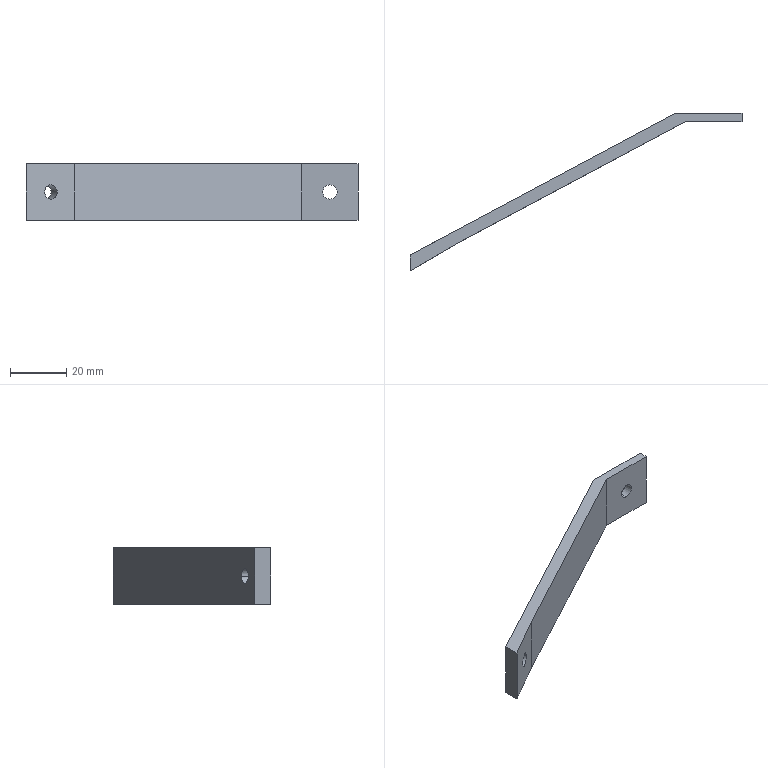Part | STEP file | Front frame | 1 solid | 13 faces | box 118.103 x 56.081 x 20 mm | volume 10734 mm3 | plane 9 | cylinder 4 | commonest cylinder face diameters 5.1 x4
STEP:
#1=CARTESIAN_POINT('',(0.,0.,0.));
#2=DIRECTION('',(0.,0.,1.));
#3=DIRECTION('',(1.,0.,0.));
#4=AXIS2_PLACEMENT_3D('',#1,#2,#3);
#5=CARTESIAN_POINT('',(-91.445,-49.238,10.));
#6=VERTEX_POINT('',#5);
#7=CARTESIAN_POINT('',(-93.677,-45.052,10.));
#8=VERTEX_POINT('',#7);
#9=CARTESIAN_POINT('',(-86.618,-58.288,10.));
#10=DIRECTION('',(-0.4706,0.8824,0.));
#11=VECTOR('',#10,1.);
#12=LINE('',#9,#11);
#13=CARTESIAN_POINT('',(-84.368,-57.088,10.));
#14=DIRECTION('',(-0.4706,0.8824,0.));
#15=DIRECTION('',(-0.8824,-0.4706,0.));
#16=AXIS2_PLACEMENT_3D('',#13,#14,#15);
#17=CYLINDRICAL_SURFACE('',#16,2.55);
#18=CARTESIAN_POINT('',(6.283,0.));
#19=DIRECTION('',(0.,1.));
#20=VECTOR('',#19,1.);
#21=LINE('',#18,#20);
#22=(GEOMETRIC_REPRESENTATION_CONTEXT(2)PARAMETRIC_REPRESENTATION_CONTEXT()REPRESENTATION_CONTEXT('',''));
#23=DEFINITIONAL_REPRESENTATION('',(#21),#22);
#24=PCURVE('',#17,#23);
#25=CARTESIAN_POINT('',(-84.368,-57.088,10.));
#26=DIRECTION('',(-0.4706,0.8824,0.));
#27=DIRECTION('',(-0.8824,-0.4706,0.));
#28=AXIS2_PLACEMENT_3D('',#25,#26,#27);
#29=CYLINDRICAL_SURFACE('',#28,2.55);
#30=CARTESIAN_POINT('',(0.,0.));
#31=DIRECTION('',(0.,1.));
#32=VECTOR('',#31,1.);
#33=LINE('',#30,#32);
#34=(GEOMETRIC_REPRESENTATION_CONTEXT(2)PARAMETRIC_REPRESENTATION_CONTEXT()REPRESENTATION_CONTEXT('',''));
#35=DEFINITIONAL_REPRESENTATION('',(#33),#34);
#36=PCURVE('',#29,#35);
#37=SURFACE_CURVE('',#12,(#24,#36),.PCURVE_S1.);
#38=EDGE_CURVE('',#6,#8,#37,.T.);
#39=ORIENTED_EDGE('',*,*,#38,.T.);
#40=CARTESIAN_POINT('',(-89.177,-42.652,10.));
#41=VERTEX_POINT('',#40);
#42=CARTESIAN_POINT('',(-91.427,-43.852,10.));
#43=DIRECTION('',(-0.4706,0.8824,0.));
#44=DIRECTION('',(-0.8824,-0.4706,0.));
#45=AXIS2_PLACEMENT_3D('',#42,#43,#44);
#46=CIRCLE('',#45,2.55);
#47=CARTESIAN_POINT('',(0.,15.));
#48=DIRECTION('',(1.,0.));
#49=VECTOR('',#48,1.);
#50=LINE('',#47,#49);
#51=(GEOMETRIC_REPRESENTATION_CONTEXT(2)PARAMETRIC_REPRESENTATION_CONTEXT()REPRESENTATION_CONTEXT('',''));
#52=DEFINITIONAL_REPRESENTATION('',(#50),#51);
#53=PCURVE('',#17,#52);
#54=CARTESIAN_POINT('',(-98.103,-47.412,133.001));
#55=DIRECTION('',(-0.4706,0.8824,0.));
#56=DIRECTION('',(-0.8824,-0.4706,0.));
#57=AXIS2_PLACEMENT_3D('',#54,#55,#56);
#58=PLANE('',#57);
#59=CARTESIAN_POINT('',(-7.566,-123.001));
#60=DIRECTION('',(1.,0.));
#61=AXIS2_PLACEMENT_2D('',#59,#60);
#62=CIRCLE('',#61,2.55);
#63=(GEOMETRIC_REPRESENTATION_CONTEXT(2)PARAMETRIC_REPRESENTATION_CONTEXT()REPRESENTATION_CONTEXT('',''));
#64=DEFINITIONAL_REPRESENTATION('',(#62),#63);
#65=PCURVE('',#58,#64);
#66=SURFACE_CURVE('',#46,(#53,#65),.PCURVE_S1.);
#67=EDGE_CURVE('',#41,#8,#66,.T.);
#68=ORIENTED_EDGE('',*,*,#67,.F.);
#69=CARTESIAN_POINT('',(-87.026,-46.686,10.));
#70=VERTEX_POINT('',#69);
#71=CARTESIAN_POINT('',(-82.118,-55.888,10.));
#72=DIRECTION('',(-0.4706,0.8824,0.));
#73=VECTOR('',#72,1.);
#74=LINE('',#71,#73);
#75=CARTESIAN_POINT('',(3.142,0.));
#76=DIRECTION('',(0.,1.));
#77=VECTOR('',#76,1.);
#78=LINE('',#75,#77);
#79=(GEOMETRIC_REPRESENTATION_CONTEXT(2)PARAMETRIC_REPRESENTATION_CONTEXT()REPRESENTATION_CONTEXT('',''));
#80=DEFINITIONAL_REPRESENTATION('',(#78),#79);
#81=PCURVE('',#17,#80);
#82=CARTESIAN_POINT('',(3.142,0.));
#83=DIRECTION('',(0.,1.));
#84=VECTOR('',#83,1.);
#85=LINE('',#82,#84);
#86=(GEOMETRIC_REPRESENTATION_CONTEXT(2)PARAMETRIC_REPRESENTATION_CONTEXT()REPRESENTATION_CONTEXT('',''));
#87=DEFINITIONAL_REPRESENTATION('',(#85),#86);
#88=PCURVE('',#29,#87);
#89=SURFACE_CURVE('',#74,(#81,#88),.PCURVE_S1.);
#90=EDGE_CURVE('',#70,#41,#89,.T.);
#91=ORIENTED_EDGE('',*,*,#90,.F.);
#92=CARTESIAN_POINT('',(-91.445,-49.238,10.));
#93=CARTESIAN_POINT('',(-91.445,-49.238,4.9));
#94=CARTESIAN_POINT('',(-87.026,-46.686,4.9));
#95=CARTESIAN_POINT('',(-87.026,-46.686,10.));
#96=(BOUNDED_CURVE()B_SPLINE_CURVE(3,(#92,#93,#94,#95),.UNSPECIFIED.,.F.,.F.)B_SPLINE_CURVE_WITH_KNOTS((4,4),(3.142,6.283),.PIECEWISE_BEZIER_KNOTS.)CURVE()GEOMETRIC_REPRESENTATION_ITEM()RATIONAL_B_SPLINE_CURVE((1.,0.3333,0.3333,1.))REPRESENTATION_ITEM(''));
#97=CARTESIAN_POINT('',(6.283,10.257));
#98=CARTESIAN_POINT('',(6.253,10.257));
#99=CARTESIAN_POINT('',(6.19,10.257));
#100=CARTESIAN_POINT('',(6.085,10.258));
#101=CARTESIAN_POINT('',(5.972,10.26));
#102=CARTESIAN_POINT('',(5.848,10.264));
#103=CARTESIAN_POINT('',(5.713,10.27));
#104=CARTESIAN_POINT('',(5.567,10.277));
#105=CARTESIAN_POINT('',(5.412,10.287));
#106=CARTESIAN_POINT('',(5.246,10.298));
#107=CARTESIAN_POINT('',(5.073,10.312));
#108=CARTESIAN_POINT('',(4.894,10.327));
#109=CARTESIAN_POINT('',(4.712,10.342));
#110=CARTESIAN_POINT('',(4.531,10.358));
#111=CARTESIAN_POINT('',(4.352,10.373));
#112=CARTESIAN_POINT('',(4.179,10.386));
#113=CARTESIAN_POINT('',(4.013,10.398));
#114=CARTESIAN_POINT('',(3.857,10.407));
#115=CARTESIAN_POINT('',(3.712,10.415));
#116=CARTESIAN_POINT('',(3.577,10.42));
#117=CARTESIAN_POINT('',(3.453,10.424));
#118=CARTESIAN_POINT('',(3.339,10.427));
#119=CARTESIAN_POINT('',(3.235,10.428));
#120=CARTESIAN_POINT('',(3.172,10.428));
#121=CARTESIAN_POINT('',(3.142,10.428));
#122=B_SPLINE_CURVE_WITH_KNOTS('',3,(#97,#98,#99,#100,#101,#102,#103,#104,#105,#106,#107,#108,#109,#110,#111,#112,#113,#114,#115,#116,#117,#118,#119,#120,#121),.UNSPECIFIED.,.F.,.F.,(4,1,1,1,1,1,1,1,1,1,1,1,1,1,1,1,1,1,1,1,1,1,4),(3.142,3.284,3.427,3.57,3.713,3.856,3.998,4.141,4.284,4.427,4.57,4.712,4.855,4.998,5.141,5.284,5.426,5.569,5.712,5.855,5.998,6.14,6.283),.QUASI_UNIFORM_KNOTS.);
#123=(GEOMETRIC_REPRESENTATION_CONTEXT(2)PARAMETRIC_REPRESENTATION_CONTEXT()REPRESENTATION_CONTEXT('',''));
#124=DEFINITIONAL_REPRESENTATION('',(#122),#123);
#125=PCURVE('',#17,#124);
#126=CARTESIAN_POINT('',(-80.782,-43.081,133.001));
#127=DIRECTION('',(0.5,-0.866,0.));
#128=DIRECTION('',(0.866,0.5,0.));
#129=AXIS2_PLACEMENT_3D('',#126,#127,#128);
#130=PLANE('',#129);
#131=CARTESIAN_POINT('',(-12.312,-123.001));
#132=CARTESIAN_POINT('',(-12.312,-128.101));
#133=CARTESIAN_POINT('',(-7.209,-128.101));
#134=CARTESIAN_POINT('',(-7.209,-123.001));
#135=(BOUNDED_CURVE()B_SPLINE_CURVE(3,(#131,#132,#133,#134),.UNSPECIFIED.,.F.,.F.)B_SPLINE_CURVE_WITH_KNOTS((4,4),(3.142,6.283),.PIECEWISE_BEZIER_KNOTS.)CURVE()GEOMETRIC_REPRESENTATION_ITEM()RATIONAL_B_SPLINE_CURVE((1.,0.3333,0.3333,1.))REPRESENTATION_ITEM(''));
#136=(GEOMETRIC_REPRESENTATION_CONTEXT(2)PARAMETRIC_REPRESENTATION_CONTEXT()REPRESENTATION_CONTEXT('',''));
#137=DEFINITIONAL_REPRESENTATION('',(#135),#136);
#138=PCURVE('',#130,#137);
#139=SURFACE_CURVE('',#96,(#125,#138),.PCURVE_S1.);
#140=EDGE_CURVE('',#6,#70,#139,.T.);
#141=ORIENTED_EDGE('',*,*,#140,.F.);
#142=EDGE_LOOP('',(#39,#68,#91,#141));
#143=FACE_BOUND('',#142,.F.);
#144=ADVANCED_FACE('',(#143),#17,.F.);
#145=CARTESIAN_POINT('',(10.,3.,7.45));
#146=VERTEX_POINT('',#145);
#147=CARTESIAN_POINT('',(10.,0.,7.45));
#148=VERTEX_POINT('',#147);
#149=CARTESIAN_POINT('',(10.,3.,7.45));
#150=DIRECTION('',(0.,-1.,0.));
#151=VECTOR('',#150,1.);
#152=LINE('',#149,#151);
#153=CARTESIAN_POINT('',(10.,3.,10.));
#154=DIRECTION('',(0.,-1.,0.));
#155=DIRECTION('',(0.,0.,-1.));
#156=AXIS2_PLACEMENT_3D('',#153,#154,#155);
#157=CYLINDRICAL_SURFACE('',#156,2.55);
#158=CARTESIAN_POINT('',(6.283,0.));
#159=DIRECTION('',(0.,1.));
#160=VECTOR('',#159,1.);
#161=LINE('',#158,#160);
#162=(GEOMETRIC_REPRESENTATION_CONTEXT(2)PARAMETRIC_REPRESENTATION_CONTEXT()REPRESENTATION_CONTEXT('',''));
#163=DEFINITIONAL_REPRESENTATION('',(#161),#162);
#164=PCURVE('',#157,#163);
#165=CARTESIAN_POINT('',(10.,3.,10.));
#166=DIRECTION('',(0.,-1.,0.));
#167=DIRECTION('',(0.,0.,-1.));
#168=AXIS2_PLACEMENT_3D('',#165,#166,#167);
#169=CYLINDRICAL_SURFACE('',#168,2.55);
#170=CARTESIAN_POINT('',(0.,0.));
#171=DIRECTION('',(0.,1.));
#172=VECTOR('',#171,1.);
#173=LINE('',#170,#172);
#174=(GEOMETRIC_REPRESENTATION_CONTEXT(2)PARAMETRIC_REPRESENTATION_CONTEXT()REPRESENTATION_CONTEXT('',''));
#175=DEFINITIONAL_REPRESENTATION('',(#173),#174);
#176=PCURVE('',#169,#175);
#177=SURFACE_CURVE('',#152,(#164,#176),.PCURVE_S1.);
#178=EDGE_CURVE('',#146,#148,#177,.T.);
#179=ORIENTED_EDGE('',*,*,#178,.T.);
#180=CARTESIAN_POINT('',(10.,0.,12.55));
#181=VERTEX_POINT('',#180);
#182=CARTESIAN_POINT('',(10.,0.,10.));
#183=DIRECTION('',(0.,1.,0.));
#184=DIRECTION('',(0.,0.,1.));
#185=AXIS2_PLACEMENT_3D('',#182,#183,#184);
#186=CIRCLE('',#185,2.55);
#187=CARTESIAN_POINT('',(9.425,3.));
#188=DIRECTION('',(-1.,0.));
#189=VECTOR('',#188,1.);
#190=LINE('',#187,#189);
#191=(GEOMETRIC_REPRESENTATION_CONTEXT(2)PARAMETRIC_REPRESENTATION_CONTEXT()REPRESENTATION_CONTEXT('',''));
#192=DEFINITIONAL_REPRESENTATION('',(#190),#191);
#193=PCURVE('',#157,#192);
#194=CARTESIAN_POINT('',(0.,0.,0.));
#195=DIRECTION('',(0.,1.,0.));
#196=DIRECTION('',(0.,0.,1.));
#197=AXIS2_PLACEMENT_3D('',#194,#195,#196);
#198=PLANE('',#197);
#199=CARTESIAN_POINT('',(10.,10.));
#200=DIRECTION('',(1.,0.));
#201=AXIS2_PLACEMENT_2D('',#199,#200);
#202=CIRCLE('',#201,2.55);
#203=(GEOMETRIC_REPRESENTATION_CONTEXT(2)PARAMETRIC_REPRESENTATION_CONTEXT()REPRESENTATION_CONTEXT('',''));
#204=DEFINITIONAL_REPRESENTATION('',(#202),#203);
#205=PCURVE('',#198,#204);
#206=SURFACE_CURVE('',#186,(#193,#205),.PCURVE_S1.);
#207=EDGE_CURVE('',#148,#181,#206,.T.);
#208=ORIENTED_EDGE('',*,*,#207,.T.);
#209=CARTESIAN_POINT('',(10.,3.,12.55));
#210=VERTEX_POINT('',#209);
#211=CARTESIAN_POINT('',(10.,3.,12.55));
#212=DIRECTION('',(0.,-1.,0.));
#213=VECTOR('',#212,1.);
#214=LINE('',#211,#213);
#215=CARTESIAN_POINT('',(3.142,0.));
#216=DIRECTION('',(0.,1.));
#217=VECTOR('',#216,1.);
#218=LINE('',#215,#217);
#219=(GEOMETRIC_REPRESENTATION_CONTEXT(2)PARAMETRIC_REPRESENTATION_CONTEXT()REPRESENTATION_CONTEXT('',''));
#220=DEFINITIONAL_REPRESENTATION('',(#218),#219);
#221=PCURVE('',#157,#220);
#222=CARTESIAN_POINT('',(3.142,0.));
#223=DIRECTION('',(0.,1.));
#224=VECTOR('',#223,1.);
#225=LINE('',#222,#224);
#226=(GEOMETRIC_REPRESENTATION_CONTEXT(2)PARAMETRIC_REPRESENTATION_CONTEXT()REPRESENTATION_CONTEXT('',''));
#227=DEFINITIONAL_REPRESENTATION('',(#225),#226);
#228=PCURVE('',#169,#227);
#229=SURFACE_CURVE('',#214,(#221,#228),.PCURVE_S1.);
#230=EDGE_CURVE('',#210,#181,#229,.T.);
#231=ORIENTED_EDGE('',*,*,#230,.F.);
#232=CARTESIAN_POINT('',(10.,3.,10.));
#233=DIRECTION('',(0.,1.,0.));
#234=DIRECTION('',(0.,0.,1.));
#235=AXIS2_PLACEMENT_3D('',#232,#233,#234);
#236=CIRCLE('',#235,2.55);
#237=CARTESIAN_POINT('',(9.425,0.));
#238=DIRECTION('',(-1.,0.));
#239=VECTOR('',#238,1.);
#240=LINE('',#237,#239);
#241=(GEOMETRIC_REPRESENTATION_CONTEXT(2)PARAMETRIC_REPRESENTATION_CONTEXT()REPRESENTATION_CONTEXT('',''));
#242=DEFINITIONAL_REPRESENTATION('',(#240),#241);
#243=PCURVE('',#157,#242);
#244=CARTESIAN_POINT('',(0.,3.,0.));
#245=DIRECTION('',(0.,1.,0.));
#246=DIRECTION('',(0.,0.,1.));
#247=AXIS2_PLACEMENT_3D('',#244,#245,#246);
#248=PLANE('',#247);
#249=CARTESIAN_POINT('',(10.,10.));
#250=DIRECTION('',(1.,0.));
#251=AXIS2_PLACEMENT_2D('',#249,#250);
#252=CIRCLE('',#251,2.55);
#253=(GEOMETRIC_REPRESENTATION_CONTEXT(2)PARAMETRIC_REPRESENTATION_CONTEXT()REPRESENTATION_CONTEXT('',''));
#254=DEFINITIONAL_REPRESENTATION('',(#252),#253);
#255=PCURVE('',#248,#254);
#256=SURFACE_CURVE('',#236,(#243,#255),.PCURVE_S1.);
#257=EDGE_CURVE('',#146,#210,#256,.T.);
#258=ORIENTED_EDGE('',*,*,#257,.F.);
#259=EDGE_LOOP('',(#179,#208,#231,#258));
#260=FACE_BOUND('',#259,.F.);
#261=ADVANCED_FACE('',(#260),#157,.F.);
#262=CARTESIAN_POINT('',(20.,3.,0.));
#263=VERTEX_POINT('',#262);
#264=CARTESIAN_POINT('',(-3.574,3.,0.));
#265=VERTEX_POINT('',#264);
#266=CARTESIAN_POINT('',(0.,3.,0.));
#267=DIRECTION('',(-1.,0.,0.));
#268=VECTOR('',#267,1.);
#269=LINE('',#266,#268);
#270=CARTESIAN_POINT('',(0.,0.));
#271=DIRECTION('',(0.,-1.));
#272=VECTOR('',#271,1.);
#273=LINE('',#270,#272);
#274=(GEOMETRIC_REPRESENTATION_CONTEXT(2)PARAMETRIC_REPRESENTATION_CONTEXT()REPRESENTATION_CONTEXT('',''));
#275=DEFINITIONAL_REPRESENTATION('',(#273),#274);
#276=PCURVE('',#248,#275);
#277=CARTESIAN_POINT('',(0.,3.,0.));
#278=DIRECTION('',(0.,0.,1.));
#279=DIRECTION('',(1.,0.,0.));
#280=AXIS2_PLACEMENT_3D('',#277,#278,#279);
#281=PLANE('',#280);
#282=CARTESIAN_POINT('',(0.,0.));
#283=DIRECTION('',(-1.,0.));
#284=VECTOR('',#283,1.);
#285=LINE('',#282,#284);
#286=(GEOMETRIC_REPRESENTATION_CONTEXT(2)PARAMETRIC_REPRESENTATION_CONTEXT()REPRESENTATION_CONTEXT('',''));
#287=DEFINITIONAL_REPRESENTATION('',(#285),#286);
#288=PCURVE('',#281,#287);
#289=SURFACE_CURVE('',#269,(#276,#288),.PCURVE_S1.);
#290=EDGE_CURVE('',#263,#265,#289,.T.);
#291=ORIENTED_EDGE('',*,*,#290,.T.);
#292=CARTESIAN_POINT('',(-3.574,3.,20.));
#293=VERTEX_POINT('',#292);
#294=CARTESIAN_POINT('',(-3.574,3.,133.001));
#295=DIRECTION('',(0.,0.,-1.));
#296=VECTOR('',#295,1.);
#297=LINE('',#294,#296);
#298=CARTESIAN_POINT('',(133.001,-3.574));
#299=DIRECTION('',(-1.,0.));
#300=VECTOR('',#299,1.);
#301=LINE('',#298,#300);
#302=(GEOMETRIC_REPRESENTATION_CONTEXT(2)PARAMETRIC_REPRESENTATION_CONTEXT()REPRESENTATION_CONTEXT('',''));
#303=DEFINITIONAL_REPRESENTATION('',(#301),#302);
#304=PCURVE('',#248,#303);
#305=CARTESIAN_POINT('',(-107.131,0.));
#306=DIRECTION('',(0.,-1.));
#307=VECTOR('',#306,1.);
#308=LINE('',#305,#307);
#309=(GEOMETRIC_REPRESENTATION_CONTEXT(2)PARAMETRIC_REPRESENTATION_CONTEXT()REPRESENTATION_CONTEXT('',''));
#310=DEFINITIONAL_REPRESENTATION('',(#308),#309);
#311=PCURVE('',#58,#310);
#312=SURFACE_CURVE('',#297,(#304,#311),.PCURVE_S1.);
#313=EDGE_CURVE('',#293,#265,#312,.T.);
#314=ORIENTED_EDGE('',*,*,#313,.F.);
#315=CARTESIAN_POINT('',(20.,3.,20.));
#316=VERTEX_POINT('',#315);
#317=CARTESIAN_POINT('',(0.,3.,20.));
#318=DIRECTION('',(1.,0.,0.));
#319=VECTOR('',#318,1.);
#320=LINE('',#317,#319);
#321=CARTESIAN_POINT('',(20.,0.));
#322=DIRECTION('',(0.,1.));
#323=VECTOR('',#322,1.);
#324=LINE('',#321,#323);
#325=(GEOMETRIC_REPRESENTATION_CONTEXT(2)PARAMETRIC_REPRESENTATION_CONTEXT()REPRESENTATION_CONTEXT('',''));
#326=DEFINITIONAL_REPRESENTATION('',(#324),#325);
#327=PCURVE('',#248,#326);
#328=CARTESIAN_POINT('',(0.,3.,20.));
#329=DIRECTION('',(0.,0.,-1.));
#330=DIRECTION('',(-1.,0.,0.));
#331=AXIS2_PLACEMENT_3D('',#328,#329,#330);
#332=PLANE('',#331);
#333=CARTESIAN_POINT('',(0.,0.));
#334=DIRECTION('',(-1.,0.));
#335=VECTOR('',#334,1.);
#336=LINE('',#333,#335);
#337=(GEOMETRIC_REPRESENTATION_CONTEXT(2)PARAMETRIC_REPRESENTATION_CONTEXT()REPRESENTATION_CONTEXT('',''));
#338=DEFINITIONAL_REPRESENTATION('',(#336),#337);
#339=PCURVE('',#332,#338);
#340=SURFACE_CURVE('',#320,(#327,#339),.PCURVE_S1.);
#341=EDGE_CURVE('',#293,#316,#340,.T.);
#342=ORIENTED_EDGE('',*,*,#341,.T.);
#343=CARTESIAN_POINT('',(20.,3.,0.));
#344=DIRECTION('',(0.,0.,-1.));
#345=VECTOR('',#344,1.);
#346=LINE('',#343,#345);
#347=CARTESIAN_POINT('',(0.,20.));
#348=DIRECTION('',(-1.,0.));
#349=VECTOR('',#348,1.);
#350=LINE('',#347,#349);
#351=(GEOMETRIC_REPRESENTATION_CONTEXT(2)PARAMETRIC_REPRESENTATION_CONTEXT()REPRESENTATION_CONTEXT('',''));
#352=DEFINITIONAL_REPRESENTATION('',(#350),#351);
#353=PCURVE('',#248,#352);
#354=CARTESIAN_POINT('',(20.,3.,0.));
#355=DIRECTION('',(-1.,0.,0.));
#356=DIRECTION('',(0.,0.,1.));
#357=AXIS2_PLACEMENT_3D('',#354,#355,#356);
#358=PLANE('',#357);
#359=CARTESIAN_POINT('',(0.,0.));
#360=DIRECTION('',(-1.,0.));
#361=VECTOR('',#360,1.);
#362=LINE('',#359,#361);
#363=(GEOMETRIC_REPRESENTATION_CONTEXT(2)PARAMETRIC_REPRESENTATION_CONTEXT()REPRESENTATION_CONTEXT('',''));
#364=DEFINITIONAL_REPRESENTATION('',(#362),#363);
#365=PCURVE('',#358,#364);
#366=SURFACE_CURVE('',#346,(#353,#365),.PCURVE_S1.);
#367=EDGE_CURVE('',#316,#263,#366,.T.);
#368=ORIENTED_EDGE('',*,*,#367,.T.);
#369=EDGE_LOOP('',(#291,#314,#342,#368));
#370=FACE_BOUND('',#369,.T.);
#371=ORIENTED_EDGE('',*,*,#257,.F.);
#372=CARTESIAN_POINT('',(10.,3.,10.));
#373=DIRECTION('',(0.,1.,0.));
#374=DIRECTION('',(0.,0.,1.));
#375=AXIS2_PLACEMENT_3D('',#372,#373,#374);
#376=CIRCLE('',#375,2.55);
#377=CARTESIAN_POINT('',(10.,10.));
#378=DIRECTION('',(1.,0.));
#379=AXIS2_PLACEMENT_2D('',#377,#378);
#380=CIRCLE('',#379,2.55);
#381=(GEOMETRIC_REPRESENTATION_CONTEXT(2)PARAMETRIC_REPRESENTATION_CONTEXT()REPRESENTATION_CONTEXT('',''));
#382=DEFINITIONAL_REPRESENTATION('',(#380),#381);
#383=PCURVE('',#248,#382);
#384=CARTESIAN_POINT('',(3.142,0.));
#385=DIRECTION('',(-1.,0.));
#386=VECTOR('',#385,1.);
#387=LINE('',#384,#386);
#388=(GEOMETRIC_REPRESENTATION_CONTEXT(2)PARAMETRIC_REPRESENTATION_CONTEXT()REPRESENTATION_CONTEXT('',''));
#389=DEFINITIONAL_REPRESENTATION('',(#387),#388);
#390=PCURVE('',#169,#389);
#391=SURFACE_CURVE('',#376,(#383,#390),.PCURVE_S1.);
#392=EDGE_CURVE('',#210,#146,#391,.T.);
#393=ORIENTED_EDGE('',*,*,#392,.F.);
#394=EDGE_LOOP('',(#371,#393));
#395=FACE_BOUND('',#394,.T.);
#396=ADVANCED_FACE('',(#370,#395),#248,.T.);
#397=CARTESIAN_POINT('',(0.,0.,0.));
#398=VERTEX_POINT('',#397);
#399=CARTESIAN_POINT('',(0.,0.,20.));
#400=VERTEX_POINT('',#399);
#401=CARTESIAN_POINT('',(0.,0.,0.));
#402=DIRECTION('',(0.,0.,1.));
#403=VECTOR('',#402,1.);
#404=LINE('',#401,#403);
#405=CARTESIAN_POINT('',(0.,0.));
#406=DIRECTION('',(1.,0.));
#407=VECTOR('',#406,1.);
#408=LINE('',#405,#407);
#409=(GEOMETRIC_REPRESENTATION_CONTEXT(2)PARAMETRIC_REPRESENTATION_CONTEXT()REPRESENTATION_CONTEXT('',''));
#410=DEFINITIONAL_REPRESENTATION('',(#408),#409);
#411=PCURVE('',#198,#410);
#412=CARTESIAN_POINT('',(0.,0.,133.001));
#413=DIRECTION('',(0.4706,-0.8824,0.));
#414=DIRECTION('',(0.8824,0.4706,0.));
#415=AXIS2_PLACEMENT_3D('',#412,#413,#414);
#416=PLANE('',#415);
#417=CARTESIAN_POINT('',(0.,-133.001));
#418=DIRECTION('',(0.,1.));
#419=VECTOR('',#418,1.);
#420=LINE('',#417,#419);
#421=(GEOMETRIC_REPRESENTATION_CONTEXT(2)PARAMETRIC_REPRESENTATION_CONTEXT()REPRESENTATION_CONTEXT('',''));
#422=DEFINITIONAL_REPRESENTATION('',(#420),#421);
#423=PCURVE('',#416,#422);
#424=SURFACE_CURVE('',#404,(#411,#423),.PCURVE_S1.);
#425=EDGE_CURVE('',#398,#400,#424,.T.);
#426=ORIENTED_EDGE('',*,*,#425,.F.);
#427=CARTESIAN_POINT('',(20.,0.,0.));
#428=VERTEX_POINT('',#427);
#429=CARTESIAN_POINT('',(0.,0.,0.));
#430=DIRECTION('',(-1.,0.,0.));
#431=VECTOR('',#430,1.);
#432=LINE('',#429,#431);
#433=CARTESIAN_POINT('',(0.,0.));
#434=DIRECTION('',(0.,-1.));
#435=VECTOR('',#434,1.);
#436=LINE('',#433,#435);
#437=(GEOMETRIC_REPRESENTATION_CONTEXT(2)PARAMETRIC_REPRESENTATION_CONTEXT()REPRESENTATION_CONTEXT('',''));
#438=DEFINITIONAL_REPRESENTATION('',(#436),#437);
#439=PCURVE('',#198,#438);
#440=CARTESIAN_POINT('',(0.,-3.));
#441=DIRECTION('',(-1.,0.));
#442=VECTOR('',#441,1.);
#443=LINE('',#440,#442);
#444=(GEOMETRIC_REPRESENTATION_CONTEXT(2)PARAMETRIC_REPRESENTATION_CONTEXT()REPRESENTATION_CONTEXT('',''));
#445=DEFINITIONAL_REPRESENTATION('',(#443),#444);
#446=PCURVE('',#281,#445);
#447=SURFACE_CURVE('',#432,(#439,#446),.PCURVE_S1.);
#448=EDGE_CURVE('',#428,#398,#447,.T.);
#449=ORIENTED_EDGE('',*,*,#448,.F.);
#450=CARTESIAN_POINT('',(20.,0.,20.));
#451=VERTEX_POINT('',#450);
#452=CARTESIAN_POINT('',(20.,0.,0.));
#453=DIRECTION('',(0.,0.,-1.));
#454=VECTOR('',#453,1.);
#455=LINE('',#452,#454);
#456=CARTESIAN_POINT('',(0.,20.));
#457=DIRECTION('',(-1.,0.));
#458=VECTOR('',#457,1.);
#459=LINE('',#456,#458);
#460=(GEOMETRIC_REPRESENTATION_CONTEXT(2)PARAMETRIC_REPRESENTATION_CONTEXT()REPRESENTATION_CONTEXT('',''));
#461=DEFINITIONAL_REPRESENTATION('',(#459),#460);
#462=PCURVE('',#198,#461);
#463=CARTESIAN_POINT('',(0.,-3.));
#464=DIRECTION('',(-1.,0.));
#465=VECTOR('',#464,1.);
#466=LINE('',#463,#465);
#467=(GEOMETRIC_REPRESENTATION_CONTEXT(2)PARAMETRIC_REPRESENTATION_CONTEXT()REPRESENTATION_CONTEXT('',''));
#468=DEFINITIONAL_REPRESENTATION('',(#466),#467);
#469=PCURVE('',#358,#468);
#470=SURFACE_CURVE('',#455,(#462,#469),.PCURVE_S1.);
#471=EDGE_CURVE('',#451,#428,#470,.T.);
#472=ORIENTED_EDGE('',*,*,#471,.F.);
#473=CARTESIAN_POINT('',(0.,0.,20.));
#474=DIRECTION('',(1.,0.,0.));
#475=VECTOR('',#474,1.);
#476=LINE('',#473,#475);
#477=CARTESIAN_POINT('',(20.,0.));
#478=DIRECTION('',(0.,1.));
#479=VECTOR('',#478,1.);
#480=LINE('',#477,#479);
#481=(GEOMETRIC_REPRESENTATION_CONTEXT(2)PARAMETRIC_REPRESENTATION_CONTEXT()REPRESENTATION_CONTEXT('',''));
#482=DEFINITIONAL_REPRESENTATION('',(#480),#481);
#483=PCURVE('',#198,#482);
#484=CARTESIAN_POINT('',(0.,-3.));
#485=DIRECTION('',(-1.,0.));
#486=VECTOR('',#485,1.);
#487=LINE('',#484,#486);
#488=(GEOMETRIC_REPRESENTATION_CONTEXT(2)PARAMETRIC_REPRESENTATION_CONTEXT()REPRESENTATION_CONTEXT('',''));
#489=DEFINITIONAL_REPRESENTATION('',(#487),#488);
#490=PCURVE('',#332,#489);
#491=SURFACE_CURVE('',#476,(#483,#490),.PCURVE_S1.);
#492=EDGE_CURVE('',#400,#451,#491,.T.);
#493=ORIENTED_EDGE('',*,*,#492,.F.);
#494=EDGE_LOOP('',(#426,#449,#472,#493));
#495=FACE_BOUND('',#494,.T.);
#496=ORIENTED_EDGE('',*,*,#207,.T.);
#497=CARTESIAN_POINT('',(10.,0.,10.));
#498=DIRECTION('',(0.,1.,0.));
#499=DIRECTION('',(0.,0.,1.));
#500=AXIS2_PLACEMENT_3D('',#497,#498,#499);
#501=CIRCLE('',#500,2.55);
#502=CARTESIAN_POINT('',(10.,10.));
#503=DIRECTION('',(1.,0.));
#504=AXIS2_PLACEMENT_2D('',#502,#503);
#505=CIRCLE('',#504,2.55);
#506=(GEOMETRIC_REPRESENTATION_CONTEXT(2)PARAMETRIC_REPRESENTATION_CONTEXT()REPRESENTATION_CONTEXT('',''));
#507=DEFINITIONAL_REPRESENTATION('',(#505),#506);
#508=PCURVE('',#198,#507);
#509=CARTESIAN_POINT('',(3.142,3.));
#510=DIRECTION('',(-1.,0.));
#511=VECTOR('',#510,1.);
#512=LINE('',#509,#511);
#513=(GEOMETRIC_REPRESENTATION_CONTEXT(2)PARAMETRIC_REPRESENTATION_CONTEXT()REPRESENTATION_CONTEXT('',''));
#514=DEFINITIONAL_REPRESENTATION('',(#512),#513);
#515=PCURVE('',#169,#514);
#516=SURFACE_CURVE('',#501,(#508,#515),.PCURVE_S1.);
#517=EDGE_CURVE('',#181,#148,#516,.T.);
#518=ORIENTED_EDGE('',*,*,#517,.T.);
#519=EDGE_LOOP('',(#496,#518));
#520=FACE_BOUND('',#519,.T.);
#521=ADVANCED_FACE('',(#495,#520),#198,.F.);
#522=ORIENTED_EDGE('',*,*,#492,.T.);
#523=CARTESIAN_POINT('',(20.,3.,20.));
#524=DIRECTION('',(0.,-1.,0.));
#525=VECTOR('',#524,1.);
#526=LINE('',#523,#525);
#527=CARTESIAN_POINT('',(-20.,0.));
#528=DIRECTION('',(0.,-1.));
#529=VECTOR('',#528,1.);
#530=LINE('',#527,#529);
#531=(GEOMETRIC_REPRESENTATION_CONTEXT(2)PARAMETRIC_REPRESENTATION_CONTEXT()REPRESENTATION_CONTEXT('',''));
#532=DEFINITIONAL_REPRESENTATION('',(#530),#531);
#533=PCURVE('',#332,#532);
#534=CARTESIAN_POINT('',(20.,0.));
#535=DIRECTION('',(0.,-1.));
#536=VECTOR('',#535,1.);
#537=LINE('',#534,#536);
#538=(GEOMETRIC_REPRESENTATION_CONTEXT(2)PARAMETRIC_REPRESENTATION_CONTEXT()REPRESENTATION_CONTEXT('',''));
#539=DEFINITIONAL_REPRESENTATION('',(#537),#538);
#540=PCURVE('',#358,#539);
#541=SURFACE_CURVE('',#526,(#533,#540),.PCURVE_S1.);
#542=EDGE_CURVE('',#316,#451,#541,.T.);
#543=ORIENTED_EDGE('',*,*,#542,.F.);
#544=ORIENTED_EDGE('',*,*,#341,.F.);
#545=CARTESIAN_POINT('',(-98.103,-47.412,20.));
#546=VERTEX_POINT('',#545);
#547=CARTESIAN_POINT('',(-98.103,-47.412,20.));
#548=DIRECTION('',(-0.8824,-0.4706,0.));
#549=VECTOR('',#548,1.);
#550=LINE('',#547,#549);
#551=CARTESIAN_POINT('',(98.103,-50.412));
#552=DIRECTION('',(0.8824,-0.4706));
#553=VECTOR('',#552,1.);
#554=LINE('',#551,#553);
#555=(GEOMETRIC_REPRESENTATION_CONTEXT(2)PARAMETRIC_REPRESENTATION_CONTEXT()REPRESENTATION_CONTEXT('',''));
#556=DEFINITIONAL_REPRESENTATION('',(#554),#555);
#557=PCURVE('',#332,#556);
#558=CARTESIAN_POINT('',(0.,-113.001));
#559=DIRECTION('',(1.,0.));
#560=VECTOR('',#559,1.);
#561=LINE('',#558,#560);
#562=(GEOMETRIC_REPRESENTATION_CONTEXT(2)PARAMETRIC_REPRESENTATION_CONTEXT()REPRESENTATION_CONTEXT('',''));
#563=DEFINITIONAL_REPRESENTATION('',(#561),#562);
#564=PCURVE('',#58,#563);
#565=SURFACE_CURVE('',#550,(#557,#564),.PCURVE_S1.);
#566=EDGE_CURVE('',#293,#546,#565,.T.);
#567=ORIENTED_EDGE('',*,*,#566,.T.);
#568=CARTESIAN_POINT('',(-98.103,-53.081,20.));
#569=VERTEX_POINT('',#568);
#570=CARTESIAN_POINT('',(-98.103,-53.081,20.));
#571=DIRECTION('',(0.,-1.,0.));
#572=VECTOR('',#571,1.);
#573=LINE('',#570,#572);
#574=CARTESIAN_POINT('',(98.103,-56.081));
#575=DIRECTION('',(0.,-1.));
#576=VECTOR('',#575,1.);
#577=LINE('',#574,#576);
#578=(GEOMETRIC_REPRESENTATION_CONTEXT(2)PARAMETRIC_REPRESENTATION_CONTEXT()REPRESENTATION_CONTEXT('',''));
#579=DEFINITIONAL_REPRESENTATION('',(#577),#578);
#580=PCURVE('',#332,#579);
#581=CARTESIAN_POINT('',(-98.103,-53.081,133.001));
#582=DIRECTION('',(-1.,0.,0.));
#583=DIRECTION('',(0.,0.,1.));
#584=AXIS2_PLACEMENT_3D('',#581,#582,#583);
#585=PLANE('',#584);
#586=CARTESIAN_POINT('',(-113.001,0.));
#587=DIRECTION('',(0.,-1.));
#588=VECTOR('',#587,1.);
#589=LINE('',#586,#588);
#590=(GEOMETRIC_REPRESENTATION_CONTEXT(2)PARAMETRIC_REPRESENTATION_CONTEXT()REPRESENTATION_CONTEXT('',''));
#591=DEFINITIONAL_REPRESENTATION('',(#589),#590);
#592=PCURVE('',#585,#591);
#593=SURFACE_CURVE('',#573,(#580,#592),.PCURVE_S1.);
#594=EDGE_CURVE('',#546,#569,#593,.T.);
#595=ORIENTED_EDGE('',*,*,#594,.T.);
#596=CARTESIAN_POINT('',(-80.782,-43.081,20.));
#597=VERTEX_POINT('',#596);
#598=CARTESIAN_POINT('',(-80.782,-43.081,20.));
#599=DIRECTION('',(0.866,0.5,0.));
#600=VECTOR('',#599,1.);
#601=LINE('',#598,#600);
#602=CARTESIAN_POINT('',(80.782,-46.081));
#603=DIRECTION('',(-0.866,0.5));
#604=VECTOR('',#603,1.);
#605=LINE('',#602,#604);
#606=(GEOMETRIC_REPRESENTATION_CONTEXT(2)PARAMETRIC_REPRESENTATION_CONTEXT()REPRESENTATION_CONTEXT('',''));
#607=DEFINITIONAL_REPRESENTATION('',(#605),#606);
#608=PCURVE('',#332,#607);
#609=CARTESIAN_POINT('',(0.,-113.001));
#610=DIRECTION('',(1.,0.));
#611=VECTOR('',#610,1.);
#612=LINE('',#609,#611);
#613=(GEOMETRIC_REPRESENTATION_CONTEXT(2)PARAMETRIC_REPRESENTATION_CONTEXT()REPRESENTATION_CONTEXT('',''));
#614=DEFINITIONAL_REPRESENTATION('',(#612),#613);
#615=PCURVE('',#130,#614);
#616=SURFACE_CURVE('',#601,(#608,#615),.PCURVE_S1.);
#617=EDGE_CURVE('',#569,#597,#616,.T.);
#618=ORIENTED_EDGE('',*,*,#617,.T.);
#619=CARTESIAN_POINT('',(0.,0.,20.));
#620=DIRECTION('',(0.8824,0.4706,0.));
#621=VECTOR('',#620,1.);
#622=LINE('',#619,#621);
#623=CARTESIAN_POINT('',(0.,-3.));
#624=DIRECTION('',(-0.8824,0.4706));
#625=VECTOR('',#624,1.);
#626=LINE('',#623,#625);
#627=(GEOMETRIC_REPRESENTATION_CONTEXT(2)PARAMETRIC_REPRESENTATION_CONTEXT()REPRESENTATION_CONTEXT('',''));
#628=DEFINITIONAL_REPRESENTATION('',(#626),#627);
#629=PCURVE('',#332,#628);
#630=CARTESIAN_POINT('',(0.,-113.001));
#631=DIRECTION('',(1.,0.));
#632=VECTOR('',#631,1.);
#633=LINE('',#630,#632);
#634=(GEOMETRIC_REPRESENTATION_CONTEXT(2)PARAMETRIC_REPRESENTATION_CONTEXT()REPRESENTATION_CONTEXT('',''));
#635=DEFINITIONAL_REPRESENTATION('',(#633),#634);
#636=PCURVE('',#416,#635);
#637=SURFACE_CURVE('',#622,(#629,#636),.PCURVE_S1.);
#638=EDGE_CURVE('',#597,#400,#637,.T.);
#639=ORIENTED_EDGE('',*,*,#638,.T.);
#640=EDGE_LOOP('',(#522,#543,#544,#567,#595,#618,#639));
#641=FACE_BOUND('',#640,.T.);
#642=ADVANCED_FACE('',(#641),#332,.F.);
#643=ORIENTED_EDGE('',*,*,#471,.T.);
#644=CARTESIAN_POINT('',(20.,3.,0.));
#645=DIRECTION('',(0.,-1.,0.));
#646=VECTOR('',#645,1.);
#647=LINE('',#644,#646);
#648=CARTESIAN_POINT('',(0.,0.));
#649=DIRECTION('',(0.,-1.));
#650=VECTOR('',#649,1.);
#651=LINE('',#648,#650);
#652=(GEOMETRIC_REPRESENTATION_CONTEXT(2)PARAMETRIC_REPRESENTATION_CONTEXT()REPRESENTATION_CONTEXT('',''));
#653=DEFINITIONAL_REPRESENTATION('',(#651),#652);
#654=PCURVE('',#358,#653);
#655=CARTESIAN_POINT('',(20.,0.));
#656=DIRECTION('',(0.,-1.));
#657=VECTOR('',#656,1.);
#658=LINE('',#655,#657);
#659=(GEOMETRIC_REPRESENTATION_CONTEXT(2)PARAMETRIC_REPRESENTATION_CONTEXT()REPRESENTATION_CONTEXT('',''));
#660=DEFINITIONAL_REPRESENTATION('',(#658),#659);
#661=PCURVE('',#281,#660);
#662=SURFACE_CURVE('',#647,(#654,#661),.PCURVE_S1.);
#663=EDGE_CURVE('',#263,#428,#662,.T.);
#664=ORIENTED_EDGE('',*,*,#663,.F.);
#665=ORIENTED_EDGE('',*,*,#367,.F.);
#666=ORIENTED_EDGE('',*,*,#542,.T.);
#667=EDGE_LOOP('',(#643,#664,#665,#666));
#668=FACE_BOUND('',#667,.T.);
#669=ADVANCED_FACE('',(#668),#358,.F.);
#670=ORIENTED_EDGE('',*,*,#448,.T.);
#671=CARTESIAN_POINT('',(-80.782,-43.081,0.));
#672=VERTEX_POINT('',#671);
#673=CARTESIAN_POINT('',(0.,0.,0.));
#674=DIRECTION('',(-0.8824,-0.4706,0.));
#675=VECTOR('',#674,1.);
#676=LINE('',#673,#675);
#677=CARTESIAN_POINT('',(0.,-3.));
#678=DIRECTION('',(-0.8824,-0.4706));
#679=VECTOR('',#678,1.);
#680=LINE('',#677,#679);
#681=(GEOMETRIC_REPRESENTATION_CONTEXT(2)PARAMETRIC_REPRESENTATION_CONTEXT()REPRESENTATION_CONTEXT('',''));
#682=DEFINITIONAL_REPRESENTATION('',(#680),#681);
#683=PCURVE('',#281,#682);
#684=CARTESIAN_POINT('',(0.,-133.001));
#685=DIRECTION('',(-1.,0.));
#686=VECTOR('',#685,1.);
#687=LINE('',#684,#686);
#688=(GEOMETRIC_REPRESENTATION_CONTEXT(2)PARAMETRIC_REPRESENTATION_CONTEXT()REPRESENTATION_CONTEXT('',''));
#689=DEFINITIONAL_REPRESENTATION('',(#687),#688);
#690=PCURVE('',#416,#689);
#691=SURFACE_CURVE('',#676,(#683,#690),.PCURVE_S1.);
#692=EDGE_CURVE('',#398,#672,#691,.T.);
#693=ORIENTED_EDGE('',*,*,#692,.T.);
#694=CARTESIAN_POINT('',(-98.103,-53.081,0.));
#695=VERTEX_POINT('',#694);
#696=CARTESIAN_POINT('',(-80.782,-43.081,0.));
#697=DIRECTION('',(-0.866,-0.5,0.));
#698=VECTOR('',#697,1.);
#699=LINE('',#696,#698);
#700=CARTESIAN_POINT('',(-80.782,-46.081));
#701=DIRECTION('',(-0.866,-0.5));
#702=VECTOR('',#701,1.);
#703=LINE('',#700,#702);
#704=(GEOMETRIC_REPRESENTATION_CONTEXT(2)PARAMETRIC_REPRESENTATION_CONTEXT()REPRESENTATION_CONTEXT('',''));
#705=DEFINITIONAL_REPRESENTATION('',(#703),#704);
#706=PCURVE('',#281,#705);
#707=CARTESIAN_POINT('',(0.,-133.001));
#708=DIRECTION('',(-1.,0.));
#709=VECTOR('',#708,1.);
#710=LINE('',#707,#709);
#711=(GEOMETRIC_REPRESENTATION_CONTEXT(2)PARAMETRIC_REPRESENTATION_CONTEXT()REPRESENTATION_CONTEXT('',''));
#712=DEFINITIONAL_REPRESENTATION('',(#710),#711);
#713=PCURVE('',#130,#712);
#714=SURFACE_CURVE('',#699,(#706,#713),.PCURVE_S1.);
#715=EDGE_CURVE('',#672,#695,#714,.T.);
#716=ORIENTED_EDGE('',*,*,#715,.T.);
#717=CARTESIAN_POINT('',(-98.103,-47.412,0.));
#718=VERTEX_POINT('',#717);
#719=CARTESIAN_POINT('',(-98.103,-53.081,0.));
#720=DIRECTION('',(0.,1.,0.));
#721=VECTOR('',#720,1.);
#722=LINE('',#719,#721);
#723=CARTESIAN_POINT('',(-98.103,-56.081));
#724=DIRECTION('',(0.,1.));
#725=VECTOR('',#724,1.);
#726=LINE('',#723,#725);
#727=(GEOMETRIC_REPRESENTATION_CONTEXT(2)PARAMETRIC_REPRESENTATION_CONTEXT()REPRESENTATION_CONTEXT('',''));
#728=DEFINITIONAL_REPRESENTATION('',(#726),#727);
#729=PCURVE('',#281,#728);
#730=CARTESIAN_POINT('',(-133.001,0.));
#731=DIRECTION('',(0.,1.));
#732=VECTOR('',#731,1.);
#733=LINE('',#730,#732);
#734=(GEOMETRIC_REPRESENTATION_CONTEXT(2)PARAMETRIC_REPRESENTATION_CONTEXT()REPRESENTATION_CONTEXT('',''));
#735=DEFINITIONAL_REPRESENTATION('',(#733),#734);
#736=PCURVE('',#585,#735);
#737=SURFACE_CURVE('',#722,(#729,#736),.PCURVE_S1.);
#738=EDGE_CURVE('',#695,#718,#737,.T.);
#739=ORIENTED_EDGE('',*,*,#738,.T.);
#740=CARTESIAN_POINT('',(-98.103,-47.412,0.));
#741=DIRECTION('',(0.8824,0.4706,0.));
#742=VECTOR('',#741,1.);
#743=LINE('',#740,#742);
#744=CARTESIAN_POINT('',(-98.103,-50.412));
#745=DIRECTION('',(0.8824,0.4706));
#746=VECTOR('',#745,1.);
#747=LINE('',#744,#746);
#748=(GEOMETRIC_REPRESENTATION_CONTEXT(2)PARAMETRIC_REPRESENTATION_CONTEXT()REPRESENTATION_CONTEXT('',''));
#749=DEFINITIONAL_REPRESENTATION('',(#747),#748);
#750=PCURVE('',#281,#749);
#751=CARTESIAN_POINT('',(0.,-133.001));
#752=DIRECTION('',(-1.,0.));
#753=VECTOR('',#752,1.);
#754=LINE('',#751,#753);
#755=(GEOMETRIC_REPRESENTATION_CONTEXT(2)PARAMETRIC_REPRESENTATION_CONTEXT()REPRESENTATION_CONTEXT('',''));
#756=DEFINITIONAL_REPRESENTATION('',(#754),#755);
#757=PCURVE('',#58,#756);
#758=SURFACE_CURVE('',#743,(#750,#757),.PCURVE_S1.);
#759=EDGE_CURVE('',#718,#265,#758,.T.);
#760=ORIENTED_EDGE('',*,*,#759,.T.);
#761=ORIENTED_EDGE('',*,*,#290,.F.);
#762=ORIENTED_EDGE('',*,*,#663,.T.);
#763=EDGE_LOOP('',(#670,#693,#716,#739,#760,#761,#762));
#764=FACE_BOUND('',#763,.T.);
#765=ADVANCED_FACE('',(#764),#281,.F.);
#766=ORIENTED_EDGE('',*,*,#517,.T.);
#767=ORIENTED_EDGE('',*,*,#178,.F.);
#768=ORIENTED_EDGE('',*,*,#392,.F.);
#769=ORIENTED_EDGE('',*,*,#230,.T.);
#770=EDGE_LOOP('',(#766,#767,#768,#769));
#771=FACE_BOUND('',#770,.F.);
#772=ADVANCED_FACE('',(#771),#169,.F.);
#773=CARTESIAN_POINT('',(-91.427,-43.852,10.));
#774=DIRECTION('',(-0.4706,0.8824,0.));
#775=DIRECTION('',(-0.8824,-0.4706,0.));
#776=AXIS2_PLACEMENT_3D('',#773,#774,#775);
#777=CIRCLE('',#776,2.55);
#778=CARTESIAN_POINT('',(-7.566,-123.001));
#779=DIRECTION('',(1.,0.));
#780=AXIS2_PLACEMENT_2D('',#778,#779);
#781=CIRCLE('',#780,2.55);
#782=(GEOMETRIC_REPRESENTATION_CONTEXT(2)PARAMETRIC_REPRESENTATION_CONTEXT()REPRESENTATION_CONTEXT('',''));
#783=DEFINITIONAL_REPRESENTATION('',(#781),#782);
#784=PCURVE('',#58,#783);
#785=CARTESIAN_POINT('',(0.,15.));
#786=DIRECTION('',(1.,0.));
#787=VECTOR('',#786,1.);
#788=LINE('',#785,#787);
#789=(GEOMETRIC_REPRESENTATION_CONTEXT(2)PARAMETRIC_REPRESENTATION_CONTEXT()REPRESENTATION_CONTEXT('',''));
#790=DEFINITIONAL_REPRESENTATION('',(#788),#789);
#791=PCURVE('',#29,#790);
#792=SURFACE_CURVE('',#777,(#784,#791),.PCURVE_S1.);
#793=EDGE_CURVE('',#8,#41,#792,.T.);
#794=ORIENTED_EDGE('',*,*,#793,.F.);
#795=ORIENTED_EDGE('',*,*,#67,.F.);
#796=EDGE_LOOP('',(#794,#795));
#797=FACE_BOUND('',#796,.T.);
#798=ORIENTED_EDGE('',*,*,#566,.F.);
#799=ORIENTED_EDGE('',*,*,#313,.T.);
#800=ORIENTED_EDGE('',*,*,#759,.F.);
#801=CARTESIAN_POINT('',(-98.103,-47.412,133.001));
#802=DIRECTION('',(0.,0.,-1.));
#803=VECTOR('',#802,1.);
#804=LINE('',#801,#803);
#805=CARTESIAN_POINT('',(0.,0.));
#806=DIRECTION('',(0.,-1.));
#807=VECTOR('',#806,1.);
#808=LINE('',#805,#807);
#809=(GEOMETRIC_REPRESENTATION_CONTEXT(2)PARAMETRIC_REPRESENTATION_CONTEXT()REPRESENTATION_CONTEXT('',''));
#810=DEFINITIONAL_REPRESENTATION('',(#808),#809);
#811=PCURVE('',#58,#810);
#812=CARTESIAN_POINT('',(0.,5.669));
#813=DIRECTION('',(-1.,0.));
#814=VECTOR('',#813,1.);
#815=LINE('',#812,#814);
#816=(GEOMETRIC_REPRESENTATION_CONTEXT(2)PARAMETRIC_REPRESENTATION_CONTEXT()REPRESENTATION_CONTEXT('',''));
#817=DEFINITIONAL_REPRESENTATION('',(#815),#816);
#818=PCURVE('',#585,#817);
#819=SURFACE_CURVE('',#804,(#811,#818),.PCURVE_S1.);
#820=EDGE_CURVE('',#546,#718,#819,.T.);
#821=ORIENTED_EDGE('',*,*,#820,.F.);
#822=EDGE_LOOP('',(#798,#799,#800,#821));
#823=FACE_BOUND('',#822,.T.);
#824=ADVANCED_FACE('',(#797,#823),#58,.T.);
#825=ORIENTED_EDGE('',*,*,#594,.F.);
#826=ORIENTED_EDGE('',*,*,#820,.T.);
#827=ORIENTED_EDGE('',*,*,#738,.F.);
#828=CARTESIAN_POINT('',(-98.103,-53.081,133.001));
#829=DIRECTION('',(0.,0.,-1.));
#830=VECTOR('',#829,1.);
#831=LINE('',#828,#830);
#832=CARTESIAN_POINT('',(0.,0.));
#833=DIRECTION('',(-1.,0.));
#834=VECTOR('',#833,1.);
#835=LINE('',#832,#834);
#836=(GEOMETRIC_REPRESENTATION_CONTEXT(2)PARAMETRIC_REPRESENTATION_CONTEXT()REPRESENTATION_CONTEXT('',''));
#837=DEFINITIONAL_REPRESENTATION('',(#835),#836);
#838=PCURVE('',#585,#837);
#839=CARTESIAN_POINT('',(-20.,0.));
#840=DIRECTION('',(0.,-1.));
#841=VECTOR('',#840,1.);
#842=LINE('',#839,#841);
#843=(GEOMETRIC_REPRESENTATION_CONTEXT(2)PARAMETRIC_REPRESENTATION_CONTEXT()REPRESENTATION_CONTEXT('',''));
#844=DEFINITIONAL_REPRESENTATION('',(#842),#843);
#845=PCURVE('',#130,#844);
#846=SURFACE_CURVE('',#831,(#838,#845),.PCURVE_S1.);
#847=EDGE_CURVE('',#569,#695,#846,.T.);
#848=ORIENTED_EDGE('',*,*,#847,.F.);
#849=EDGE_LOOP('',(#825,#826,#827,#848));
#850=FACE_BOUND('',#849,.T.);
#851=ADVANCED_FACE('',(#850),#585,.T.);
#852=ORIENTED_EDGE('',*,*,#140,.F.);
#853=CARTESIAN_POINT('',(-87.026,-46.686,10.));
#854=CARTESIAN_POINT('',(-87.026,-46.686,15.1));
#855=CARTESIAN_POINT('',(-91.445,-49.238,15.1));
#856=CARTESIAN_POINT('',(-91.445,-49.238,10.));
#857=(BOUNDED_CURVE()B_SPLINE_CURVE(3,(#853,#854,#855,#856),.UNSPECIFIED.,.F.,.F.)B_SPLINE_CURVE_WITH_KNOTS((4,4),(0.,3.142),.PIECEWISE_BEZIER_KNOTS.)CURVE()GEOMETRIC_REPRESENTATION_ITEM()RATIONAL_B_SPLINE_CURVE((1.,0.3333,0.3333,1.))REPRESENTATION_ITEM(''));
#858=CARTESIAN_POINT('',(-7.209,-123.001));
#859=CARTESIAN_POINT('',(-7.209,-117.901));
#860=CARTESIAN_POINT('',(-12.312,-117.901));
#861=CARTESIAN_POINT('',(-12.312,-123.001));
#862=(BOUNDED_CURVE()B_SPLINE_CURVE(3,(#858,#859,#860,#861),.UNSPECIFIED.,.F.,.F.)B_SPLINE_CURVE_WITH_KNOTS((4,4),(0.,3.142),.PIECEWISE_BEZIER_KNOTS.)CURVE()GEOMETRIC_REPRESENTATION_ITEM()RATIONAL_B_SPLINE_CURVE((1.,0.3333,0.3333,1.))REPRESENTATION_ITEM(''));
#863=(GEOMETRIC_REPRESENTATION_CONTEXT(2)PARAMETRIC_REPRESENTATION_CONTEXT()REPRESENTATION_CONTEXT('',''));
#864=DEFINITIONAL_REPRESENTATION('',(#862),#863);
#865=PCURVE('',#130,#864);
#866=CARTESIAN_POINT('',(3.142,10.428));
#867=CARTESIAN_POINT('',(3.111,10.428));
#868=CARTESIAN_POINT('',(3.048,10.428));
#869=CARTESIAN_POINT('',(2.944,10.427));
#870=CARTESIAN_POINT('',(2.83,10.424));
#871=CARTESIAN_POINT('',(2.706,10.42));
#872=CARTESIAN_POINT('',(2.571,10.415));
#873=CARTESIAN_POINT('',(2.426,10.407));
#874=CARTESIAN_POINT('',(2.27,10.398));
#875=CARTESIAN_POINT('',(2.105,10.386));
#876=CARTESIAN_POINT('',(1.931,10.373));
#877=CARTESIAN_POINT('',(1.753,10.358));
#878=CARTESIAN_POINT('',(1.571,10.342));
#879=CARTESIAN_POINT('',(1.389,10.327));
#880=CARTESIAN_POINT('',(1.21,10.312));
#881=CARTESIAN_POINT('',(1.037,10.298));
#882=CARTESIAN_POINT('',(0.8717,10.287));
#883=CARTESIAN_POINT('',(0.7158,10.277));
#884=CARTESIAN_POINT('',(0.5703,10.27));
#885=CARTESIAN_POINT('',(0.4356,10.264));
#886=CARTESIAN_POINT('',(0.3115,10.26));
#887=CARTESIAN_POINT('',(0.1977,10.258));
#888=CARTESIAN_POINT('',(0.09367,10.257));
#889=CARTESIAN_POINT('',(0.0303,10.257));
#890=CARTESIAN_POINT('',(0.,10.257));
#891=B_SPLINE_CURVE_WITH_KNOTS('',3,(#866,#867,#868,#869,#870,#871,#872,#873,#874,#875,#876,#877,#878,#879,#880,#881,#882,#883,#884,#885,#886,#887,#888,#889,#890),.UNSPECIFIED.,.F.,.F.,(4,1,1,1,1,1,1,1,1,1,1,1,1,1,1,1,1,1,1,1,1,1,4),(0.,0.1428,0.2856,0.4284,0.5712,0.714,0.8568,0.9996,1.142,1.285,1.428,1.571,1.714,1.856,1.999,2.142,2.285,2.428,2.57,2.713,2.856,2.999,3.142),.QUASI_UNIFORM_KNOTS.);
#892=(GEOMETRIC_REPRESENTATION_CONTEXT(2)PARAMETRIC_REPRESENTATION_CONTEXT()REPRESENTATION_CONTEXT('',''));
#893=DEFINITIONAL_REPRESENTATION('',(#891),#892);
#894=PCURVE('',#29,#893);
#895=SURFACE_CURVE('',#857,(#865,#894),.PCURVE_S1.);
#896=EDGE_CURVE('',#70,#6,#895,.T.);
#897=ORIENTED_EDGE('',*,*,#896,.F.);
#898=EDGE_LOOP('',(#852,#897));
#899=FACE_BOUND('',#898,.T.);
#900=ORIENTED_EDGE('',*,*,#617,.F.);
#901=ORIENTED_EDGE('',*,*,#847,.T.);
#902=ORIENTED_EDGE('',*,*,#715,.F.);
#903=CARTESIAN_POINT('',(-80.782,-43.081,133.001));
#904=DIRECTION('',(0.,0.,-1.));
#905=VECTOR('',#904,1.);
#906=LINE('',#903,#905);
#907=CARTESIAN_POINT('',(0.,0.));
#908=DIRECTION('',(0.,-1.));
#909=VECTOR('',#908,1.);
#910=LINE('',#907,#909);
#911=(GEOMETRIC_REPRESENTATION_CONTEXT(2)PARAMETRIC_REPRESENTATION_CONTEXT()REPRESENTATION_CONTEXT('',''));
#912=DEFINITIONAL_REPRESENTATION('',(#910),#911);
#913=PCURVE('',#130,#912);
#914=CARTESIAN_POINT('',(-91.552,0.));
#915=DIRECTION('',(0.,-1.));
#916=VECTOR('',#915,1.);
#917=LINE('',#914,#916);
#918=(GEOMETRIC_REPRESENTATION_CONTEXT(2)PARAMETRIC_REPRESENTATION_CONTEXT()REPRESENTATION_CONTEXT('',''));
#919=DEFINITIONAL_REPRESENTATION('',(#917),#918);
#920=PCURVE('',#416,#919);
#921=SURFACE_CURVE('',#906,(#913,#920),.PCURVE_S1.);
#922=EDGE_CURVE('',#597,#672,#921,.T.);
#923=ORIENTED_EDGE('',*,*,#922,.F.);
#924=EDGE_LOOP('',(#900,#901,#902,#923));
#925=FACE_BOUND('',#924,.T.);
#926=ADVANCED_FACE('',(#899,#925),#130,.T.);
#927=ORIENTED_EDGE('',*,*,#638,.F.);
#928=ORIENTED_EDGE('',*,*,#922,.T.);
#929=ORIENTED_EDGE('',*,*,#692,.F.);
#930=ORIENTED_EDGE('',*,*,#425,.T.);
#931=EDGE_LOOP('',(#927,#928,#929,#930));
#932=FACE_BOUND('',#931,.T.);
#933=ADVANCED_FACE('',(#932),#416,.T.);
#934=ORIENTED_EDGE('',*,*,#793,.F.);
#935=ORIENTED_EDGE('',*,*,#38,.F.);
#936=ORIENTED_EDGE('',*,*,#896,.F.);
#937=ORIENTED_EDGE('',*,*,#90,.T.);
#938=EDGE_LOOP('',(#934,#935,#936,#937));
#939=FACE_BOUND('',#938,.F.);
#940=ADVANCED_FACE('',(#939),#29,.F.);
#941=CLOSED_SHELL('',(#144,#261,#396,#521,#642,#669,#765,#772,#824,#851,#926,#933,#940));
#942=MANIFOLD_SOLID_BREP('',#941);
#943=(LENGTH_UNIT()NAMED_UNIT(*)SI_UNIT(.MILLI.,.METRE.));
#944=UNCERTAINTY_MEASURE_WITH_UNIT(LENGTH_MEASURE(0.0000001),#943,'','');
#945=(NAMED_UNIT(*)PLANE_ANGLE_UNIT()SI_UNIT($,.RADIAN.));
#946=(NAMED_UNIT(*)SI_UNIT($,.STERADIAN.)SOLID_ANGLE_UNIT());
#947=(GEOMETRIC_REPRESENTATION_CONTEXT(3)GLOBAL_UNCERTAINTY_ASSIGNED_CONTEXT((#944))GLOBAL_UNIT_ASSIGNED_CONTEXT((#943,#945,#946))REPRESENTATION_CONTEXT('',''));
#948=ADVANCED_BREP_SHAPE_REPRESENTATION('',(#4,#942),#947);